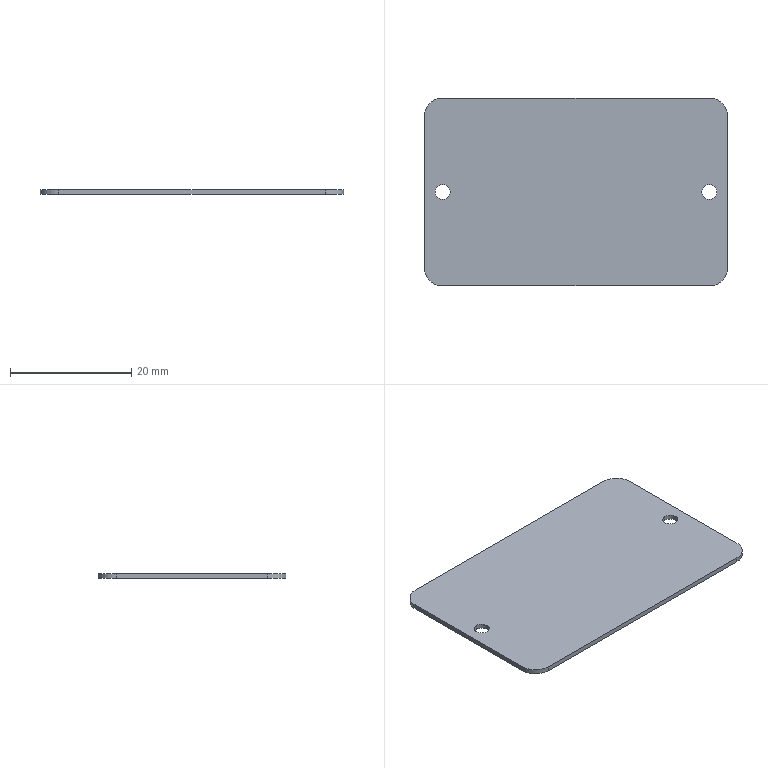Part | STEP file | Grease nameplate-Part-2 | 1 solid | 14 faces | box 50 x 31 x 0.8 mm | volume 1226 mm3 | cylinder 8 | plane 6 | commonest cylinder face diameters 2.5 x4 6 x4
STEP:
#1=CARTESIAN_POINT('',(0.,0.,0.));
#2=DIRECTION('',(0.,0.,1.));
#3=DIRECTION('',(1.,0.,0.));
#4=AXIS2_PLACEMENT_3D('',#1,#2,#3);
#5=CARTESIAN_POINT('',(47.,-16.75,0.8));
#6=VERTEX_POINT('',#5);
#7=CARTESIAN_POINT('',(47.,-16.75,0.));
#8=VERTEX_POINT('',#7);
#9=CARTESIAN_POINT('',(47.,-16.75,0.8));
#10=DIRECTION('',(0.,0.,-1.));
#11=VECTOR('',#10,1.);
#12=LINE('',#9,#11);
#13=CARTESIAN_POINT('',(47.,-15.5,0.8));
#14=DIRECTION('',(0.,0.,-1.));
#15=DIRECTION('',(0.,-1.,0.));
#16=AXIS2_PLACEMENT_3D('',#13,#14,#15);
#17=CYLINDRICAL_SURFACE('',#16,1.25);
#18=CARTESIAN_POINT('',(6.283,0.));
#19=DIRECTION('',(0.,1.));
#20=VECTOR('',#19,1.);
#21=LINE('',#18,#20);
#22=(GEOMETRIC_REPRESENTATION_CONTEXT(2)PARAMETRIC_REPRESENTATION_CONTEXT()REPRESENTATION_CONTEXT('',''));
#23=DEFINITIONAL_REPRESENTATION('',(#21),#22);
#24=PCURVE('',#17,#23);
#25=CARTESIAN_POINT('',(47.,-15.5,0.8));
#26=DIRECTION('',(0.,0.,-1.));
#27=DIRECTION('',(0.,-1.,0.));
#28=AXIS2_PLACEMENT_3D('',#25,#26,#27);
#29=CYLINDRICAL_SURFACE('',#28,1.25);
#30=CARTESIAN_POINT('',(0.,0.));
#31=DIRECTION('',(0.,1.));
#32=VECTOR('',#31,1.);
#33=LINE('',#30,#32);
#34=(GEOMETRIC_REPRESENTATION_CONTEXT(2)PARAMETRIC_REPRESENTATION_CONTEXT()REPRESENTATION_CONTEXT('',''));
#35=DEFINITIONAL_REPRESENTATION('',(#33),#34);
#36=PCURVE('',#29,#35);
#37=SURFACE_CURVE('',#12,(#24,#36),.PCURVE_S1.);
#38=EDGE_CURVE('',#6,#8,#37,.T.);
#39=ORIENTED_EDGE('',*,*,#38,.T.);
#40=CARTESIAN_POINT('',(47.,-14.25,0.));
#41=VERTEX_POINT('',#40);
#42=CARTESIAN_POINT('',(47.,-15.5,0.));
#43=DIRECTION('',(0.,0.,-1.));
#44=DIRECTION('',(0.,1.,0.));
#45=AXIS2_PLACEMENT_3D('',#42,#43,#44);
#46=CIRCLE('',#45,1.25);
#47=CARTESIAN_POINT('',(3.142,0.8));
#48=DIRECTION('',(1.,0.));
#49=VECTOR('',#48,1.);
#50=LINE('',#47,#49);
#51=(GEOMETRIC_REPRESENTATION_CONTEXT(2)PARAMETRIC_REPRESENTATION_CONTEXT()REPRESENTATION_CONTEXT('',''));
#52=DEFINITIONAL_REPRESENTATION('',(#50),#51);
#53=PCURVE('',#17,#52);
#54=CARTESIAN_POINT('',(25.,0.,0.));
#55=DIRECTION('',(0.,0.,-1.));
#56=DIRECTION('',(0.,-1.,0.));
#57=AXIS2_PLACEMENT_3D('',#54,#55,#56);
#58=PLANE('',#57);
#59=CARTESIAN_POINT('',(15.5,-22.));
#60=DIRECTION('',(-1.,0.));
#61=AXIS2_PLACEMENT_2D('',#59,#60);
#62=CIRCLE('',#61,1.25);
#63=(GEOMETRIC_REPRESENTATION_CONTEXT(2)PARAMETRIC_REPRESENTATION_CONTEXT()REPRESENTATION_CONTEXT('',''));
#64=DEFINITIONAL_REPRESENTATION('',(#62),#63);
#65=PCURVE('',#58,#64);
#66=SURFACE_CURVE('',#46,(#53,#65),.PCURVE_S1.);
#67=EDGE_CURVE('',#41,#8,#66,.T.);
#68=ORIENTED_EDGE('',*,*,#67,.F.);
#69=CARTESIAN_POINT('',(47.,-14.25,0.8));
#70=VERTEX_POINT('',#69);
#71=CARTESIAN_POINT('',(47.,-14.25,0.8));
#72=DIRECTION('',(0.,0.,-1.));
#73=VECTOR('',#72,1.);
#74=LINE('',#71,#73);
#75=CARTESIAN_POINT('',(3.142,0.));
#76=DIRECTION('',(0.,1.));
#77=VECTOR('',#76,1.);
#78=LINE('',#75,#77);
#79=(GEOMETRIC_REPRESENTATION_CONTEXT(2)PARAMETRIC_REPRESENTATION_CONTEXT()REPRESENTATION_CONTEXT('',''));
#80=DEFINITIONAL_REPRESENTATION('',(#78),#79);
#81=PCURVE('',#17,#80);
#82=CARTESIAN_POINT('',(3.142,0.));
#83=DIRECTION('',(0.,1.));
#84=VECTOR('',#83,1.);
#85=LINE('',#82,#84);
#86=(GEOMETRIC_REPRESENTATION_CONTEXT(2)PARAMETRIC_REPRESENTATION_CONTEXT()REPRESENTATION_CONTEXT('',''));
#87=DEFINITIONAL_REPRESENTATION('',(#85),#86);
#88=PCURVE('',#29,#87);
#89=SURFACE_CURVE('',#74,(#81,#88),.PCURVE_S1.);
#90=EDGE_CURVE('',#70,#41,#89,.T.);
#91=ORIENTED_EDGE('',*,*,#90,.F.);
#92=CARTESIAN_POINT('',(47.,-15.5,0.8));
#93=DIRECTION('',(0.,0.,1.));
#94=DIRECTION('',(0.,-1.,0.));
#95=AXIS2_PLACEMENT_3D('',#92,#93,#94);
#96=CIRCLE('',#95,1.25);
#97=CARTESIAN_POINT('',(6.283,0.));
#98=DIRECTION('',(-1.,0.));
#99=VECTOR('',#98,1.);
#100=LINE('',#97,#99);
#101=(GEOMETRIC_REPRESENTATION_CONTEXT(2)PARAMETRIC_REPRESENTATION_CONTEXT()REPRESENTATION_CONTEXT('',''));
#102=DEFINITIONAL_REPRESENTATION('',(#100),#101);
#103=PCURVE('',#17,#102);
#104=CARTESIAN_POINT('',(25.,0.,0.8));
#105=DIRECTION('',(0.,0.,1.));
#106=DIRECTION('',(0.,1.,0.));
#107=AXIS2_PLACEMENT_3D('',#104,#105,#106);
#108=PLANE('',#107);
#109=CARTESIAN_POINT('',(-15.5,-22.));
#110=DIRECTION('',(-1.,0.));
#111=AXIS2_PLACEMENT_2D('',#109,#110);
#112=CIRCLE('',#111,1.25);
#113=(GEOMETRIC_REPRESENTATION_CONTEXT(2)PARAMETRIC_REPRESENTATION_CONTEXT()REPRESENTATION_CONTEXT('',''));
#114=DEFINITIONAL_REPRESENTATION('',(#112),#113);
#115=PCURVE('',#108,#114);
#116=SURFACE_CURVE('',#96,(#103,#115),.PCURVE_S1.);
#117=EDGE_CURVE('',#6,#70,#116,.T.);
#118=ORIENTED_EDGE('',*,*,#117,.F.);
#119=EDGE_LOOP('',(#39,#68,#91,#118));
#120=FACE_BOUND('',#119,.F.);
#121=ADVANCED_FACE('',(#120),#17,.F.);
#122=CARTESIAN_POINT('',(3.,-16.75,0.8));
#123=VERTEX_POINT('',#122);
#124=CARTESIAN_POINT('',(3.,-16.75,0.));
#125=VERTEX_POINT('',#124);
#126=CARTESIAN_POINT('',(3.,-16.75,0.8));
#127=DIRECTION('',(0.,0.,-1.));
#128=VECTOR('',#127,1.);
#129=LINE('',#126,#128);
#130=CARTESIAN_POINT('',(3.,-15.5,0.8));
#131=DIRECTION('',(0.,0.,-1.));
#132=DIRECTION('',(0.,-1.,0.));
#133=AXIS2_PLACEMENT_3D('',#130,#131,#132);
#134=CYLINDRICAL_SURFACE('',#133,1.25);
#135=CARTESIAN_POINT('',(6.283,0.));
#136=DIRECTION('',(0.,1.));
#137=VECTOR('',#136,1.);
#138=LINE('',#135,#137);
#139=(GEOMETRIC_REPRESENTATION_CONTEXT(2)PARAMETRIC_REPRESENTATION_CONTEXT()REPRESENTATION_CONTEXT('',''));
#140=DEFINITIONAL_REPRESENTATION('',(#138),#139);
#141=PCURVE('',#134,#140);
#142=CARTESIAN_POINT('',(3.,-15.5,0.8));
#143=DIRECTION('',(0.,0.,-1.));
#144=DIRECTION('',(0.,-1.,0.));
#145=AXIS2_PLACEMENT_3D('',#142,#143,#144);
#146=CYLINDRICAL_SURFACE('',#145,1.25);
#147=CARTESIAN_POINT('',(0.,0.));
#148=DIRECTION('',(0.,1.));
#149=VECTOR('',#148,1.);
#150=LINE('',#147,#149);
#151=(GEOMETRIC_REPRESENTATION_CONTEXT(2)PARAMETRIC_REPRESENTATION_CONTEXT()REPRESENTATION_CONTEXT('',''));
#152=DEFINITIONAL_REPRESENTATION('',(#150),#151);
#153=PCURVE('',#146,#152);
#154=SURFACE_CURVE('',#129,(#141,#153),.PCURVE_S1.);
#155=EDGE_CURVE('',#123,#125,#154,.T.);
#156=ORIENTED_EDGE('',*,*,#155,.T.);
#157=CARTESIAN_POINT('',(3.,-14.25,0.));
#158=VERTEX_POINT('',#157);
#159=CARTESIAN_POINT('',(3.,-15.5,0.));
#160=DIRECTION('',(0.,0.,-1.));
#161=DIRECTION('',(0.,1.,0.));
#162=AXIS2_PLACEMENT_3D('',#159,#160,#161);
#163=CIRCLE('',#162,1.25);
#164=CARTESIAN_POINT('',(3.142,0.8));
#165=DIRECTION('',(1.,0.));
#166=VECTOR('',#165,1.);
#167=LINE('',#164,#166);
#168=(GEOMETRIC_REPRESENTATION_CONTEXT(2)PARAMETRIC_REPRESENTATION_CONTEXT()REPRESENTATION_CONTEXT('',''));
#169=DEFINITIONAL_REPRESENTATION('',(#167),#168);
#170=PCURVE('',#134,#169);
#171=CARTESIAN_POINT('',(15.5,22.));
#172=DIRECTION('',(-1.,0.));
#173=AXIS2_PLACEMENT_2D('',#171,#172);
#174=CIRCLE('',#173,1.25);
#175=(GEOMETRIC_REPRESENTATION_CONTEXT(2)PARAMETRIC_REPRESENTATION_CONTEXT()REPRESENTATION_CONTEXT('',''));
#176=DEFINITIONAL_REPRESENTATION('',(#174),#175);
#177=PCURVE('',#58,#176);
#178=SURFACE_CURVE('',#163,(#170,#177),.PCURVE_S1.);
#179=EDGE_CURVE('',#158,#125,#178,.T.);
#180=ORIENTED_EDGE('',*,*,#179,.F.);
#181=CARTESIAN_POINT('',(3.,-14.25,0.8));
#182=VERTEX_POINT('',#181);
#183=CARTESIAN_POINT('',(3.,-14.25,0.8));
#184=DIRECTION('',(0.,0.,-1.));
#185=VECTOR('',#184,1.);
#186=LINE('',#183,#185);
#187=CARTESIAN_POINT('',(3.142,0.));
#188=DIRECTION('',(0.,1.));
#189=VECTOR('',#188,1.);
#190=LINE('',#187,#189);
#191=(GEOMETRIC_REPRESENTATION_CONTEXT(2)PARAMETRIC_REPRESENTATION_CONTEXT()REPRESENTATION_CONTEXT('',''));
#192=DEFINITIONAL_REPRESENTATION('',(#190),#191);
#193=PCURVE('',#134,#192);
#194=CARTESIAN_POINT('',(3.142,0.));
#195=DIRECTION('',(0.,1.));
#196=VECTOR('',#195,1.);
#197=LINE('',#194,#196);
#198=(GEOMETRIC_REPRESENTATION_CONTEXT(2)PARAMETRIC_REPRESENTATION_CONTEXT()REPRESENTATION_CONTEXT('',''));
#199=DEFINITIONAL_REPRESENTATION('',(#197),#198);
#200=PCURVE('',#146,#199);
#201=SURFACE_CURVE('',#186,(#193,#200),.PCURVE_S1.);
#202=EDGE_CURVE('',#182,#158,#201,.T.);
#203=ORIENTED_EDGE('',*,*,#202,.F.);
#204=CARTESIAN_POINT('',(3.,-15.5,0.8));
#205=DIRECTION('',(0.,0.,1.));
#206=DIRECTION('',(0.,-1.,0.));
#207=AXIS2_PLACEMENT_3D('',#204,#205,#206);
#208=CIRCLE('',#207,1.25);
#209=CARTESIAN_POINT('',(6.283,0.));
#210=DIRECTION('',(-1.,0.));
#211=VECTOR('',#210,1.);
#212=LINE('',#209,#211);
#213=(GEOMETRIC_REPRESENTATION_CONTEXT(2)PARAMETRIC_REPRESENTATION_CONTEXT()REPRESENTATION_CONTEXT('',''));
#214=DEFINITIONAL_REPRESENTATION('',(#212),#213);
#215=PCURVE('',#134,#214);
#216=CARTESIAN_POINT('',(-15.5,22.));
#217=DIRECTION('',(-1.,0.));
#218=AXIS2_PLACEMENT_2D('',#216,#217);
#219=CIRCLE('',#218,1.25);
#220=(GEOMETRIC_REPRESENTATION_CONTEXT(2)PARAMETRIC_REPRESENTATION_CONTEXT()REPRESENTATION_CONTEXT('',''));
#221=DEFINITIONAL_REPRESENTATION('',(#219),#220);
#222=PCURVE('',#108,#221);
#223=SURFACE_CURVE('',#208,(#215,#222),.PCURVE_S1.);
#224=EDGE_CURVE('',#123,#182,#223,.T.);
#225=ORIENTED_EDGE('',*,*,#224,.F.);
#226=EDGE_LOOP('',(#156,#180,#203,#225));
#227=FACE_BOUND('',#226,.F.);
#228=ADVANCED_FACE('',(#227),#134,.F.);
#229=CARTESIAN_POINT('',(3.,-31.,0.));
#230=VERTEX_POINT('',#229);
#231=CARTESIAN_POINT('',(47.,-31.,0.));
#232=VERTEX_POINT('',#231);
#233=CARTESIAN_POINT('',(25.,-31.,0.));
#234=DIRECTION('',(1.,0.,0.));
#235=VECTOR('',#234,1.);
#236=LINE('',#233,#235);
#237=CARTESIAN_POINT('',(25.,-31.,0.4));
#238=DIRECTION('',(0.,-1.,0.));
#239=DIRECTION('',(1.,0.,0.));
#240=AXIS2_PLACEMENT_3D('',#237,#238,#239);
#241=PLANE('',#240);
#242=CARTESIAN_POINT('',(0.,-0.4));
#243=DIRECTION('',(1.,0.));
#244=VECTOR('',#243,1.);
#245=LINE('',#242,#244);
#246=(GEOMETRIC_REPRESENTATION_CONTEXT(2)PARAMETRIC_REPRESENTATION_CONTEXT()REPRESENTATION_CONTEXT('',''));
#247=DEFINITIONAL_REPRESENTATION('',(#245),#246);
#248=PCURVE('',#241,#247);
#249=CARTESIAN_POINT('',(31.,0.));
#250=DIRECTION('',(0.,-1.));
#251=VECTOR('',#250,1.);
#252=LINE('',#249,#251);
#253=(GEOMETRIC_REPRESENTATION_CONTEXT(2)PARAMETRIC_REPRESENTATION_CONTEXT()REPRESENTATION_CONTEXT('',''));
#254=DEFINITIONAL_REPRESENTATION('',(#252),#253);
#255=PCURVE('',#58,#254);
#256=SURFACE_CURVE('',#236,(#248,#255),.PCURVE_S1.);
#257=EDGE_CURVE('',#230,#232,#256,.T.);
#258=ORIENTED_EDGE('',*,*,#257,.T.);
#259=CARTESIAN_POINT('',(47.,-31.,0.8));
#260=VERTEX_POINT('',#259);
#261=CARTESIAN_POINT('',(47.,-31.,0.4));
#262=DIRECTION('',(0.,0.,-1.));
#263=VECTOR('',#262,1.);
#264=LINE('',#261,#263);
#265=CARTESIAN_POINT('',(22.,0.));
#266=DIRECTION('',(0.,-1.));
#267=VECTOR('',#266,1.);
#268=LINE('',#265,#267);
#269=(GEOMETRIC_REPRESENTATION_CONTEXT(2)PARAMETRIC_REPRESENTATION_CONTEXT()REPRESENTATION_CONTEXT('',''));
#270=DEFINITIONAL_REPRESENTATION('',(#268),#269);
#271=PCURVE('',#241,#270);
#272=CARTESIAN_POINT('',(47.,-28.,0.4));
#273=DIRECTION('',(0.,0.,1.));
#274=DIRECTION('',(0.,1.,0.));
#275=AXIS2_PLACEMENT_3D('',#272,#273,#274);
#276=CYLINDRICAL_SURFACE('',#275,3.);
#277=CARTESIAN_POINT('',(3.142,0.));
#278=DIRECTION('',(0.,-1.));
#279=VECTOR('',#278,1.);
#280=LINE('',#277,#279);
#281=(GEOMETRIC_REPRESENTATION_CONTEXT(2)PARAMETRIC_REPRESENTATION_CONTEXT()REPRESENTATION_CONTEXT('',''));
#282=DEFINITIONAL_REPRESENTATION('',(#280),#281);
#283=PCURVE('',#276,#282);
#284=SURFACE_CURVE('',#264,(#271,#283),.PCURVE_S1.);
#285=EDGE_CURVE('',#260,#232,#284,.T.);
#286=ORIENTED_EDGE('',*,*,#285,.F.);
#287=CARTESIAN_POINT('',(3.,-31.,0.8));
#288=VERTEX_POINT('',#287);
#289=CARTESIAN_POINT('',(25.,-31.,0.8));
#290=DIRECTION('',(-1.,0.,0.));
#291=VECTOR('',#290,1.);
#292=LINE('',#289,#291);
#293=CARTESIAN_POINT('',(0.,0.4));
#294=DIRECTION('',(-1.,0.));
#295=VECTOR('',#294,1.);
#296=LINE('',#293,#295);
#297=(GEOMETRIC_REPRESENTATION_CONTEXT(2)PARAMETRIC_REPRESENTATION_CONTEXT()REPRESENTATION_CONTEXT('',''));
#298=DEFINITIONAL_REPRESENTATION('',(#296),#297);
#299=PCURVE('',#241,#298);
#300=CARTESIAN_POINT('',(-31.,0.));
#301=DIRECTION('',(0.,1.));
#302=VECTOR('',#301,1.);
#303=LINE('',#300,#302);
#304=(GEOMETRIC_REPRESENTATION_CONTEXT(2)PARAMETRIC_REPRESENTATION_CONTEXT()REPRESENTATION_CONTEXT('',''));
#305=DEFINITIONAL_REPRESENTATION('',(#303),#304);
#306=PCURVE('',#108,#305);
#307=SURFACE_CURVE('',#292,(#299,#306),.PCURVE_S1.);
#308=EDGE_CURVE('',#260,#288,#307,.T.);
#309=ORIENTED_EDGE('',*,*,#308,.T.);
#310=CARTESIAN_POINT('',(3.,-31.,0.4));
#311=DIRECTION('',(0.,0.,1.));
#312=VECTOR('',#311,1.);
#313=LINE('',#310,#312);
#314=CARTESIAN_POINT('',(-22.,0.));
#315=DIRECTION('',(0.,1.));
#316=VECTOR('',#315,1.);
#317=LINE('',#314,#316);
#318=(GEOMETRIC_REPRESENTATION_CONTEXT(2)PARAMETRIC_REPRESENTATION_CONTEXT()REPRESENTATION_CONTEXT('',''));
#319=DEFINITIONAL_REPRESENTATION('',(#317),#318);
#320=PCURVE('',#241,#319);
#321=CARTESIAN_POINT('',(3.,-28.,0.4));
#322=DIRECTION('',(0.,0.,-1.));
#323=DIRECTION('',(0.,-1.,0.));
#324=AXIS2_PLACEMENT_3D('',#321,#322,#323);
#325=CYLINDRICAL_SURFACE('',#324,3.);
#326=CARTESIAN_POINT('',(0.,0.));
#327=DIRECTION('',(0.,-1.));
#328=VECTOR('',#327,1.);
#329=LINE('',#326,#328);
#330=(GEOMETRIC_REPRESENTATION_CONTEXT(2)PARAMETRIC_REPRESENTATION_CONTEXT()REPRESENTATION_CONTEXT('',''));
#331=DEFINITIONAL_REPRESENTATION('',(#329),#330);
#332=PCURVE('',#325,#331);
#333=SURFACE_CURVE('',#313,(#320,#332),.PCURVE_S1.);
#334=EDGE_CURVE('',#230,#288,#333,.T.);
#335=ORIENTED_EDGE('',*,*,#334,.F.);
#336=EDGE_LOOP('',(#258,#286,#309,#335));
#337=FACE_BOUND('',#336,.T.);
#338=ADVANCED_FACE('',(#337),#241,.T.);
#339=ORIENTED_EDGE('',*,*,#117,.F.);
#340=CARTESIAN_POINT('',(47.,-15.5,0.8));
#341=DIRECTION('',(0.,0.,1.));
#342=DIRECTION('',(0.,-1.,0.));
#343=AXIS2_PLACEMENT_3D('',#340,#341,#342);
#344=CIRCLE('',#343,1.25);
#345=CARTESIAN_POINT('',(-15.5,-22.));
#346=DIRECTION('',(-1.,0.));
#347=AXIS2_PLACEMENT_2D('',#345,#346);
#348=CIRCLE('',#347,1.25);
#349=(GEOMETRIC_REPRESENTATION_CONTEXT(2)PARAMETRIC_REPRESENTATION_CONTEXT()REPRESENTATION_CONTEXT('',''));
#350=DEFINITIONAL_REPRESENTATION('',(#348),#349);
#351=PCURVE('',#108,#350);
#352=CARTESIAN_POINT('',(6.283,0.));
#353=DIRECTION('',(-1.,0.));
#354=VECTOR('',#353,1.);
#355=LINE('',#352,#354);
#356=(GEOMETRIC_REPRESENTATION_CONTEXT(2)PARAMETRIC_REPRESENTATION_CONTEXT()REPRESENTATION_CONTEXT('',''));
#357=DEFINITIONAL_REPRESENTATION('',(#355),#356);
#358=PCURVE('',#29,#357);
#359=SURFACE_CURVE('',#344,(#351,#358),.PCURVE_S1.);
#360=EDGE_CURVE('',#70,#6,#359,.T.);
#361=ORIENTED_EDGE('',*,*,#360,.F.);
#362=EDGE_LOOP('',(#339,#361));
#363=FACE_BOUND('',#362,.T.);
#364=ORIENTED_EDGE('',*,*,#224,.F.);
#365=CARTESIAN_POINT('',(3.,-15.5,0.8));
#366=DIRECTION('',(0.,0.,1.));
#367=DIRECTION('',(0.,-1.,0.));
#368=AXIS2_PLACEMENT_3D('',#365,#366,#367);
#369=CIRCLE('',#368,1.25);
#370=CARTESIAN_POINT('',(-15.5,22.));
#371=DIRECTION('',(-1.,0.));
#372=AXIS2_PLACEMENT_2D('',#370,#371);
#373=CIRCLE('',#372,1.25);
#374=(GEOMETRIC_REPRESENTATION_CONTEXT(2)PARAMETRIC_REPRESENTATION_CONTEXT()REPRESENTATION_CONTEXT('',''));
#375=DEFINITIONAL_REPRESENTATION('',(#373),#374);
#376=PCURVE('',#108,#375);
#377=CARTESIAN_POINT('',(6.283,0.));
#378=DIRECTION('',(-1.,0.));
#379=VECTOR('',#378,1.);
#380=LINE('',#377,#379);
#381=(GEOMETRIC_REPRESENTATION_CONTEXT(2)PARAMETRIC_REPRESENTATION_CONTEXT()REPRESENTATION_CONTEXT('',''));
#382=DEFINITIONAL_REPRESENTATION('',(#380),#381);
#383=PCURVE('',#146,#382);
#384=SURFACE_CURVE('',#369,(#376,#383),.PCURVE_S1.);
#385=EDGE_CURVE('',#182,#123,#384,.T.);
#386=ORIENTED_EDGE('',*,*,#385,.F.);
#387=EDGE_LOOP('',(#364,#386));
#388=FACE_BOUND('',#387,.T.);
#389=CARTESIAN_POINT('',(0.,-3.,0.8));
#390=VERTEX_POINT('',#389);
#391=CARTESIAN_POINT('',(0.,-28.,0.8));
#392=VERTEX_POINT('',#391);
#393=CARTESIAN_POINT('',(0.,0.,0.8));
#394=DIRECTION('',(0.,-1.,0.));
#395=VECTOR('',#394,1.);
#396=LINE('',#393,#395);
#397=CARTESIAN_POINT('',(0.,25.));
#398=DIRECTION('',(-1.,0.));
#399=VECTOR('',#398,1.);
#400=LINE('',#397,#399);
#401=(GEOMETRIC_REPRESENTATION_CONTEXT(2)PARAMETRIC_REPRESENTATION_CONTEXT()REPRESENTATION_CONTEXT('',''));
#402=DEFINITIONAL_REPRESENTATION('',(#400),#401);
#403=PCURVE('',#108,#402);
#404=CARTESIAN_POINT('',(0.,0.,0.4));
#405=DIRECTION('',(-1.,0.,0.));
#406=DIRECTION('',(0.,-1.,0.));
#407=AXIS2_PLACEMENT_3D('',#404,#405,#406);
#408=PLANE('',#407);
#409=CARTESIAN_POINT('',(0.,0.4));
#410=DIRECTION('',(1.,0.));
#411=VECTOR('',#410,1.);
#412=LINE('',#409,#411);
#413=(GEOMETRIC_REPRESENTATION_CONTEXT(2)PARAMETRIC_REPRESENTATION_CONTEXT()REPRESENTATION_CONTEXT('',''));
#414=DEFINITIONAL_REPRESENTATION('',(#412),#413);
#415=PCURVE('',#408,#414);
#416=SURFACE_CURVE('',#396,(#403,#415),.PCURVE_S1.);
#417=EDGE_CURVE('',#390,#392,#416,.T.);
#418=ORIENTED_EDGE('',*,*,#417,.T.);
#419=CARTESIAN_POINT('',(3.,-28.,0.8));
#420=DIRECTION('',(0.,0.,-1.));
#421=DIRECTION('',(0.,1.,0.));
#422=AXIS2_PLACEMENT_3D('',#419,#420,#421);
#423=CIRCLE('',#422,3.);
#424=CARTESIAN_POINT('',(-25.,22.));
#425=CARTESIAN_POINT('',(-25.,16.804));
#426=CARTESIAN_POINT('',(-29.5,19.402));
#427=CARTESIAN_POINT('',(-34.,22.));
#428=CARTESIAN_POINT('',(-29.5,24.598));
#429=CARTESIAN_POINT('',(-25.,27.196));
#430=CARTESIAN_POINT('',(-25.,22.));
#431=(BOUNDED_CURVE()B_SPLINE_CURVE(2,(#424,#425,#426,#427,#428,#429,#430),.UNSPECIFIED.,.T.,.F.)B_SPLINE_CURVE_WITH_KNOTS((1,2,2,2,2,1),(-2.094,0.,2.094,4.189,6.283,8.378),.UNSPECIFIED.)CURVE()GEOMETRIC_REPRESENTATION_ITEM()RATIONAL_B_SPLINE_CURVE((1.,0.5,1.,0.5,1.,0.5,1.))REPRESENTATION_ITEM(''));
#432=(GEOMETRIC_REPRESENTATION_CONTEXT(2)PARAMETRIC_REPRESENTATION_CONTEXT()REPRESENTATION_CONTEXT('',''));
#433=DEFINITIONAL_REPRESENTATION('',(#431),#432);
#434=PCURVE('',#108,#433);
#435=CARTESIAN_POINT('',(-3.142,-0.4));
#436=DIRECTION('',(1.,0.));
#437=VECTOR('',#436,1.);
#438=LINE('',#435,#437);
#439=(GEOMETRIC_REPRESENTATION_CONTEXT(2)PARAMETRIC_REPRESENTATION_CONTEXT()REPRESENTATION_CONTEXT('',''));
#440=DEFINITIONAL_REPRESENTATION('',(#438),#439);
#441=PCURVE('',#325,#440);
#442=SURFACE_CURVE('',#423,(#434,#441),.PCURVE_S1.);
#443=EDGE_CURVE('',#288,#392,#442,.T.);
#444=ORIENTED_EDGE('',*,*,#443,.F.);
#445=ORIENTED_EDGE('',*,*,#308,.F.);
#446=CARTESIAN_POINT('',(50.,-28.,0.8));
#447=VERTEX_POINT('',#446);
#448=CARTESIAN_POINT('',(47.,-28.,0.8));
#449=DIRECTION('',(0.,0.,-1.));
#450=DIRECTION('',(0.,1.,0.));
#451=AXIS2_PLACEMENT_3D('',#448,#449,#450);
#452=CIRCLE('',#451,3.);
#453=CARTESIAN_POINT('',(-25.,-22.));
#454=CARTESIAN_POINT('',(-25.,-27.196));
#455=CARTESIAN_POINT('',(-29.5,-24.598));
#456=CARTESIAN_POINT('',(-34.,-22.));
#457=CARTESIAN_POINT('',(-29.5,-19.402));
#458=CARTESIAN_POINT('',(-25.,-16.804));
#459=CARTESIAN_POINT('',(-25.,-22.));
#460=(BOUNDED_CURVE()B_SPLINE_CURVE(2,(#453,#454,#455,#456,#457,#458,#459),.UNSPECIFIED.,.T.,.F.)B_SPLINE_CURVE_WITH_KNOTS((1,2,2,2,2,1),(-2.094,0.,2.094,4.189,6.283,8.378),.UNSPECIFIED.)CURVE()GEOMETRIC_REPRESENTATION_ITEM()RATIONAL_B_SPLINE_CURVE((1.,0.5,1.,0.5,1.,0.5,1.))REPRESENTATION_ITEM(''));
#461=(GEOMETRIC_REPRESENTATION_CONTEXT(2)PARAMETRIC_REPRESENTATION_CONTEXT()REPRESENTATION_CONTEXT('',''));
#462=DEFINITIONAL_REPRESENTATION('',(#460),#461);
#463=PCURVE('',#108,#462);
#464=CARTESIAN_POINT('',(6.283,0.4));
#465=DIRECTION('',(-1.,0.));
#466=VECTOR('',#465,1.);
#467=LINE('',#464,#466);
#468=(GEOMETRIC_REPRESENTATION_CONTEXT(2)PARAMETRIC_REPRESENTATION_CONTEXT()REPRESENTATION_CONTEXT('',''));
#469=DEFINITIONAL_REPRESENTATION('',(#467),#468);
#470=PCURVE('',#276,#469);
#471=SURFACE_CURVE('',#452,(#463,#470),.PCURVE_S1.);
#472=EDGE_CURVE('',#447,#260,#471,.T.);
#473=ORIENTED_EDGE('',*,*,#472,.F.);
#474=CARTESIAN_POINT('',(50.,-3.,0.8));
#475=VERTEX_POINT('',#474);
#476=CARTESIAN_POINT('',(50.,0.,0.8));
#477=DIRECTION('',(0.,-1.,0.));
#478=VECTOR('',#477,1.);
#479=LINE('',#476,#478);
#480=CARTESIAN_POINT('',(0.,-25.));
#481=DIRECTION('',(-1.,0.));
#482=VECTOR('',#481,1.);
#483=LINE('',#480,#482);
#484=(GEOMETRIC_REPRESENTATION_CONTEXT(2)PARAMETRIC_REPRESENTATION_CONTEXT()REPRESENTATION_CONTEXT('',''));
#485=DEFINITIONAL_REPRESENTATION('',(#483),#484);
#486=PCURVE('',#108,#485);
#487=CARTESIAN_POINT('',(50.,0.,0.4));
#488=DIRECTION('',(1.,0.,0.));
#489=DIRECTION('',(0.,1.,0.));
#490=AXIS2_PLACEMENT_3D('',#487,#488,#489);
#491=PLANE('',#490);
#492=CARTESIAN_POINT('',(0.,0.4));
#493=DIRECTION('',(-1.,0.));
#494=VECTOR('',#493,1.);
#495=LINE('',#492,#494);
#496=(GEOMETRIC_REPRESENTATION_CONTEXT(2)PARAMETRIC_REPRESENTATION_CONTEXT()REPRESENTATION_CONTEXT('',''));
#497=DEFINITIONAL_REPRESENTATION('',(#495),#496);
#498=PCURVE('',#491,#497);
#499=SURFACE_CURVE('',#479,(#486,#498),.PCURVE_S1.);
#500=EDGE_CURVE('',#475,#447,#499,.T.);
#501=ORIENTED_EDGE('',*,*,#500,.F.);
#502=CARTESIAN_POINT('',(47.,0.,0.8));
#503=VERTEX_POINT('',#502);
#504=CARTESIAN_POINT('',(47.,-3.,0.8));
#505=DIRECTION('',(0.,0.,-1.));
#506=DIRECTION('',(0.,1.,0.));
#507=AXIS2_PLACEMENT_3D('',#504,#505,#506);
#508=CIRCLE('',#507,3.);
#509=CARTESIAN_POINT('',(0.,-22.));
#510=CARTESIAN_POINT('',(0.,-27.196));
#511=CARTESIAN_POINT('',(-4.5,-24.598));
#512=CARTESIAN_POINT('',(-9.,-22.));
#513=CARTESIAN_POINT('',(-4.5,-19.402));
#514=CARTESIAN_POINT('',(0.,-16.804));
#515=CARTESIAN_POINT('',(0.,-22.));
#516=(BOUNDED_CURVE()B_SPLINE_CURVE(2,(#509,#510,#511,#512,#513,#514,#515),.UNSPECIFIED.,.T.,.F.)B_SPLINE_CURVE_WITH_KNOTS((1,2,2,2,2,1),(-2.094,0.,2.094,4.189,6.283,8.378),.UNSPECIFIED.)CURVE()GEOMETRIC_REPRESENTATION_ITEM()RATIONAL_B_SPLINE_CURVE((1.,0.5,1.,0.5,1.,0.5,1.))REPRESENTATION_ITEM(''));
#517=(GEOMETRIC_REPRESENTATION_CONTEXT(2)PARAMETRIC_REPRESENTATION_CONTEXT()REPRESENTATION_CONTEXT('',''));
#518=DEFINITIONAL_REPRESENTATION('',(#516),#517);
#519=PCURVE('',#108,#518);
#520=CARTESIAN_POINT('',(47.,-3.,0.4));
#521=DIRECTION('',(0.,0.,-1.));
#522=DIRECTION('',(0.,-1.,0.));
#523=AXIS2_PLACEMENT_3D('',#520,#521,#522);
#524=CYLINDRICAL_SURFACE('',#523,3.);
#525=CARTESIAN_POINT('',(3.142,-0.4));
#526=DIRECTION('',(1.,0.));
#527=VECTOR('',#526,1.);
#528=LINE('',#525,#527);
#529=(GEOMETRIC_REPRESENTATION_CONTEXT(2)PARAMETRIC_REPRESENTATION_CONTEXT()REPRESENTATION_CONTEXT('',''));
#530=DEFINITIONAL_REPRESENTATION('',(#528),#529);
#531=PCURVE('',#524,#530);
#532=SURFACE_CURVE('',#508,(#519,#531),.PCURVE_S1.);
#533=EDGE_CURVE('',#503,#475,#532,.T.);
#534=ORIENTED_EDGE('',*,*,#533,.F.);
#535=CARTESIAN_POINT('',(3.,0.,0.8));
#536=VERTEX_POINT('',#535);
#537=CARTESIAN_POINT('',(25.,0.,0.8));
#538=DIRECTION('',(1.,0.,0.));
#539=VECTOR('',#538,1.);
#540=LINE('',#537,#539);
#541=CARTESIAN_POINT('',(0.,0.));
#542=DIRECTION('',(0.,-1.));
#543=VECTOR('',#542,1.);
#544=LINE('',#541,#543);
#545=(GEOMETRIC_REPRESENTATION_CONTEXT(2)PARAMETRIC_REPRESENTATION_CONTEXT()REPRESENTATION_CONTEXT('',''));
#546=DEFINITIONAL_REPRESENTATION('',(#544),#545);
#547=PCURVE('',#108,#546);
#548=CARTESIAN_POINT('',(25.,0.,0.4));
#549=DIRECTION('',(0.,1.,0.));
#550=DIRECTION('',(-1.,0.,0.));
#551=AXIS2_PLACEMENT_3D('',#548,#549,#550);
#552=PLANE('',#551);
#553=CARTESIAN_POINT('',(0.,0.4));
#554=DIRECTION('',(-1.,0.));
#555=VECTOR('',#554,1.);
#556=LINE('',#553,#555);
#557=(GEOMETRIC_REPRESENTATION_CONTEXT(2)PARAMETRIC_REPRESENTATION_CONTEXT()REPRESENTATION_CONTEXT('',''));
#558=DEFINITIONAL_REPRESENTATION('',(#556),#557);
#559=PCURVE('',#552,#558);
#560=SURFACE_CURVE('',#540,(#547,#559),.PCURVE_S1.);
#561=EDGE_CURVE('',#536,#503,#560,.T.);
#562=ORIENTED_EDGE('',*,*,#561,.F.);
#563=CARTESIAN_POINT('',(3.,-3.,0.8));
#564=DIRECTION('',(0.,0.,-1.));
#565=DIRECTION('',(0.,1.,0.));
#566=AXIS2_PLACEMENT_3D('',#563,#564,#565);
#567=CIRCLE('',#566,3.);
#568=CARTESIAN_POINT('',(0.,22.));
#569=CARTESIAN_POINT('',(0.,16.804));
#570=CARTESIAN_POINT('',(-4.5,19.402));
#571=CARTESIAN_POINT('',(-9.,22.));
#572=CARTESIAN_POINT('',(-4.5,24.598));
#573=CARTESIAN_POINT('',(0.,27.196));
#574=CARTESIAN_POINT('',(0.,22.));
#575=(BOUNDED_CURVE()B_SPLINE_CURVE(2,(#568,#569,#570,#571,#572,#573,#574),.UNSPECIFIED.,.T.,.F.)B_SPLINE_CURVE_WITH_KNOTS((1,2,2,2,2,1),(-2.094,0.,2.094,4.189,6.283,8.378),.UNSPECIFIED.)CURVE()GEOMETRIC_REPRESENTATION_ITEM()RATIONAL_B_SPLINE_CURVE((1.,0.5,1.,0.5,1.,0.5,1.))REPRESENTATION_ITEM(''));
#576=(GEOMETRIC_REPRESENTATION_CONTEXT(2)PARAMETRIC_REPRESENTATION_CONTEXT()REPRESENTATION_CONTEXT('',''));
#577=DEFINITIONAL_REPRESENTATION('',(#575),#576);
#578=PCURVE('',#108,#577);
#579=CARTESIAN_POINT('',(3.,-3.,0.4));
#580=DIRECTION('',(0.,0.,1.));
#581=DIRECTION('',(0.,1.,0.));
#582=AXIS2_PLACEMENT_3D('',#579,#580,#581);
#583=CYLINDRICAL_SURFACE('',#582,3.);
#584=CARTESIAN_POINT('',(6.283,0.4));
#585=DIRECTION('',(-1.,0.));
#586=VECTOR('',#585,1.);
#587=LINE('',#584,#586);
#588=(GEOMETRIC_REPRESENTATION_CONTEXT(2)PARAMETRIC_REPRESENTATION_CONTEXT()REPRESENTATION_CONTEXT('',''));
#589=DEFINITIONAL_REPRESENTATION('',(#587),#588);
#590=PCURVE('',#583,#589);
#591=SURFACE_CURVE('',#567,(#578,#590),.PCURVE_S1.);
#592=EDGE_CURVE('',#390,#536,#591,.T.);
#593=ORIENTED_EDGE('',*,*,#592,.F.);
#594=EDGE_LOOP('',(#418,#444,#445,#473,#501,#534,#562,#593));
#595=FACE_BOUND('',#594,.T.);
#596=ADVANCED_FACE('',(#363,#388,#595),#108,.T.);
#597=CARTESIAN_POINT('',(0.,-3.,0.));
#598=VERTEX_POINT('',#597);
#599=CARTESIAN_POINT('',(0.,-28.,0.));
#600=VERTEX_POINT('',#599);
#601=CARTESIAN_POINT('',(0.,0.,0.));
#602=DIRECTION('',(0.,-1.,0.));
#603=VECTOR('',#602,1.);
#604=LINE('',#601,#603);
#605=CARTESIAN_POINT('',(0.,-0.4));
#606=DIRECTION('',(1.,0.));
#607=VECTOR('',#606,1.);
#608=LINE('',#605,#607);
#609=(GEOMETRIC_REPRESENTATION_CONTEXT(2)PARAMETRIC_REPRESENTATION_CONTEXT()REPRESENTATION_CONTEXT('',''));
#610=DEFINITIONAL_REPRESENTATION('',(#608),#609);
#611=PCURVE('',#408,#610);
#612=CARTESIAN_POINT('',(0.,25.));
#613=DIRECTION('',(1.,0.));
#614=VECTOR('',#613,1.);
#615=LINE('',#612,#614);
#616=(GEOMETRIC_REPRESENTATION_CONTEXT(2)PARAMETRIC_REPRESENTATION_CONTEXT()REPRESENTATION_CONTEXT('',''));
#617=DEFINITIONAL_REPRESENTATION('',(#615),#616);
#618=PCURVE('',#58,#617);
#619=SURFACE_CURVE('',#604,(#611,#618),.PCURVE_S1.);
#620=EDGE_CURVE('',#598,#600,#619,.T.);
#621=ORIENTED_EDGE('',*,*,#620,.T.);
#622=CARTESIAN_POINT('',(0.,-28.,0.4));
#623=DIRECTION('',(0.,0.,-1.));
#624=VECTOR('',#623,1.);
#625=LINE('',#622,#624);
#626=CARTESIAN_POINT('',(28.,0.));
#627=DIRECTION('',(0.,-1.));
#628=VECTOR('',#627,1.);
#629=LINE('',#626,#628);
#630=(GEOMETRIC_REPRESENTATION_CONTEXT(2)PARAMETRIC_REPRESENTATION_CONTEXT()REPRESENTATION_CONTEXT('',''));
#631=DEFINITIONAL_REPRESENTATION('',(#629),#630);
#632=PCURVE('',#408,#631);
#633=CARTESIAN_POINT('',(1.571,0.));
#634=DIRECTION('',(0.,1.));
#635=VECTOR('',#634,1.);
#636=LINE('',#633,#635);
#637=(GEOMETRIC_REPRESENTATION_CONTEXT(2)PARAMETRIC_REPRESENTATION_CONTEXT()REPRESENTATION_CONTEXT('',''));
#638=DEFINITIONAL_REPRESENTATION('',(#636),#637);
#639=PCURVE('',#325,#638);
#640=SURFACE_CURVE('',#625,(#632,#639),.PCURVE_S1.);
#641=EDGE_CURVE('',#392,#600,#640,.T.);
#642=ORIENTED_EDGE('',*,*,#641,.F.);
#643=ORIENTED_EDGE('',*,*,#417,.F.);
#644=CARTESIAN_POINT('',(0.,-3.,0.4));
#645=DIRECTION('',(0.,0.,1.));
#646=VECTOR('',#645,1.);
#647=LINE('',#644,#646);
#648=CARTESIAN_POINT('',(3.,0.));
#649=DIRECTION('',(0.,1.));
#650=VECTOR('',#649,1.);
#651=LINE('',#648,#650);
#652=(GEOMETRIC_REPRESENTATION_CONTEXT(2)PARAMETRIC_REPRESENTATION_CONTEXT()REPRESENTATION_CONTEXT('',''));
#653=DEFINITIONAL_REPRESENTATION('',(#651),#652);
#654=PCURVE('',#408,#653);
#655=CARTESIAN_POINT('',(1.571,0.));
#656=DIRECTION('',(0.,1.));
#657=VECTOR('',#656,1.);
#658=LINE('',#655,#657);
#659=(GEOMETRIC_REPRESENTATION_CONTEXT(2)PARAMETRIC_REPRESENTATION_CONTEXT()REPRESENTATION_CONTEXT('',''));
#660=DEFINITIONAL_REPRESENTATION('',(#658),#659);
#661=PCURVE('',#583,#660);
#662=SURFACE_CURVE('',#647,(#654,#661),.PCURVE_S1.);
#663=EDGE_CURVE('',#598,#390,#662,.T.);
#664=ORIENTED_EDGE('',*,*,#663,.F.);
#665=EDGE_LOOP('',(#621,#642,#643,#664));
#666=FACE_BOUND('',#665,.T.);
#667=ADVANCED_FACE('',(#666),#408,.T.);
#668=CARTESIAN_POINT('',(47.,-15.5,0.));
#669=DIRECTION('',(0.,0.,-1.));
#670=DIRECTION('',(0.,1.,0.));
#671=AXIS2_PLACEMENT_3D('',#668,#669,#670);
#672=CIRCLE('',#671,1.25);
#673=CARTESIAN_POINT('',(15.5,-22.));
#674=DIRECTION('',(-1.,0.));
#675=AXIS2_PLACEMENT_2D('',#673,#674);
#676=CIRCLE('',#675,1.25);
#677=(GEOMETRIC_REPRESENTATION_CONTEXT(2)PARAMETRIC_REPRESENTATION_CONTEXT()REPRESENTATION_CONTEXT('',''));
#678=DEFINITIONAL_REPRESENTATION('',(#676),#677);
#679=PCURVE('',#58,#678);
#680=CARTESIAN_POINT('',(-3.142,0.8));
#681=DIRECTION('',(1.,0.));
#682=VECTOR('',#681,1.);
#683=LINE('',#680,#682);
#684=(GEOMETRIC_REPRESENTATION_CONTEXT(2)PARAMETRIC_REPRESENTATION_CONTEXT()REPRESENTATION_CONTEXT('',''));
#685=DEFINITIONAL_REPRESENTATION('',(#683),#684);
#686=PCURVE('',#29,#685);
#687=SURFACE_CURVE('',#672,(#679,#686),.PCURVE_S1.);
#688=EDGE_CURVE('',#8,#41,#687,.T.);
#689=ORIENTED_EDGE('',*,*,#688,.F.);
#690=ORIENTED_EDGE('',*,*,#67,.F.);
#691=EDGE_LOOP('',(#689,#690));
#692=FACE_BOUND('',#691,.T.);
#693=CARTESIAN_POINT('',(3.,-15.5,0.));
#694=DIRECTION('',(0.,0.,-1.));
#695=DIRECTION('',(0.,1.,0.));
#696=AXIS2_PLACEMENT_3D('',#693,#694,#695);
#697=CIRCLE('',#696,1.25);
#698=CARTESIAN_POINT('',(15.5,22.));
#699=DIRECTION('',(-1.,0.));
#700=AXIS2_PLACEMENT_2D('',#698,#699);
#701=CIRCLE('',#700,1.25);
#702=(GEOMETRIC_REPRESENTATION_CONTEXT(2)PARAMETRIC_REPRESENTATION_CONTEXT()REPRESENTATION_CONTEXT('',''));
#703=DEFINITIONAL_REPRESENTATION('',(#701),#702);
#704=PCURVE('',#58,#703);
#705=CARTESIAN_POINT('',(-3.142,0.8));
#706=DIRECTION('',(1.,0.));
#707=VECTOR('',#706,1.);
#708=LINE('',#705,#707);
#709=(GEOMETRIC_REPRESENTATION_CONTEXT(2)PARAMETRIC_REPRESENTATION_CONTEXT()REPRESENTATION_CONTEXT('',''));
#710=DEFINITIONAL_REPRESENTATION('',(#708),#709);
#711=PCURVE('',#146,#710);
#712=SURFACE_CURVE('',#697,(#704,#711),.PCURVE_S1.);
#713=EDGE_CURVE('',#125,#158,#712,.T.);
#714=ORIENTED_EDGE('',*,*,#713,.F.);
#715=ORIENTED_EDGE('',*,*,#179,.F.);
#716=EDGE_LOOP('',(#714,#715));
#717=FACE_BOUND('',#716,.T.);
#718=CARTESIAN_POINT('',(47.,0.,0.));
#719=VERTEX_POINT('',#718);
#720=CARTESIAN_POINT('',(3.,0.,0.));
#721=VERTEX_POINT('',#720);
#722=CARTESIAN_POINT('',(25.,0.,0.));
#723=DIRECTION('',(-1.,0.,0.));
#724=VECTOR('',#723,1.);
#725=LINE('',#722,#724);
#726=CARTESIAN_POINT('',(0.,0.));
#727=DIRECTION('',(0.,1.));
#728=VECTOR('',#727,1.);
#729=LINE('',#726,#728);
#730=(GEOMETRIC_REPRESENTATION_CONTEXT(2)PARAMETRIC_REPRESENTATION_CONTEXT()REPRESENTATION_CONTEXT('',''));
#731=DEFINITIONAL_REPRESENTATION('',(#729),#730);
#732=PCURVE('',#58,#731);
#733=CARTESIAN_POINT('',(0.,-0.4));
#734=DIRECTION('',(1.,0.));
#735=VECTOR('',#734,1.);
#736=LINE('',#733,#735);
#737=(GEOMETRIC_REPRESENTATION_CONTEXT(2)PARAMETRIC_REPRESENTATION_CONTEXT()REPRESENTATION_CONTEXT('',''));
#738=DEFINITIONAL_REPRESENTATION('',(#736),#737);
#739=PCURVE('',#552,#738);
#740=SURFACE_CURVE('',#725,(#732,#739),.PCURVE_S1.);
#741=EDGE_CURVE('',#719,#721,#740,.T.);
#742=ORIENTED_EDGE('',*,*,#741,.F.);
#743=CARTESIAN_POINT('',(50.,-3.,0.));
#744=VERTEX_POINT('',#743);
#745=CARTESIAN_POINT('',(47.,-3.,0.));
#746=DIRECTION('',(0.,0.,1.));
#747=DIRECTION('',(0.,-1.,0.));
#748=AXIS2_PLACEMENT_3D('',#745,#746,#747);
#749=CIRCLE('',#748,3.);
#750=CARTESIAN_POINT('',(6.,-22.));
#751=CARTESIAN_POINT('',(6.,-27.196));
#752=CARTESIAN_POINT('',(1.5,-24.598));
#753=CARTESIAN_POINT('',(-3.,-22.));
#754=CARTESIAN_POINT('',(1.5,-19.402));
#755=CARTESIAN_POINT('',(6.,-16.804));
#756=CARTESIAN_POINT('',(6.,-22.));
#757=(BOUNDED_CURVE()B_SPLINE_CURVE(2,(#750,#751,#752,#753,#754,#755,#756),.UNSPECIFIED.,.T.,.F.)B_SPLINE_CURVE_WITH_KNOTS((1,2,2,2,2,1),(-2.094,0.,2.094,4.189,6.283,8.378),.UNSPECIFIED.)CURVE()GEOMETRIC_REPRESENTATION_ITEM()RATIONAL_B_SPLINE_CURVE((1.,0.5,1.,0.5,1.,0.5,1.))REPRESENTATION_ITEM(''));
#758=(GEOMETRIC_REPRESENTATION_CONTEXT(2)PARAMETRIC_REPRESENTATION_CONTEXT()REPRESENTATION_CONTEXT('',''));
#759=DEFINITIONAL_REPRESENTATION('',(#757),#758);
#760=PCURVE('',#58,#759);
#761=CARTESIAN_POINT('',(6.283,0.4));
#762=DIRECTION('',(-1.,0.));
#763=VECTOR('',#762,1.);
#764=LINE('',#761,#763);
#765=(GEOMETRIC_REPRESENTATION_CONTEXT(2)PARAMETRIC_REPRESENTATION_CONTEXT()REPRESENTATION_CONTEXT('',''));
#766=DEFINITIONAL_REPRESENTATION('',(#764),#765);
#767=PCURVE('',#524,#766);
#768=SURFACE_CURVE('',#749,(#760,#767),.PCURVE_S1.);
#769=EDGE_CURVE('',#744,#719,#768,.T.);
#770=ORIENTED_EDGE('',*,*,#769,.F.);
#771=CARTESIAN_POINT('',(50.,-28.,0.));
#772=VERTEX_POINT('',#771);
#773=CARTESIAN_POINT('',(50.,0.,0.));
#774=DIRECTION('',(0.,-1.,0.));
#775=VECTOR('',#774,1.);
#776=LINE('',#773,#775);
#777=CARTESIAN_POINT('',(0.,-25.));
#778=DIRECTION('',(1.,0.));
#779=VECTOR('',#778,1.);
#780=LINE('',#777,#779);
#781=(GEOMETRIC_REPRESENTATION_CONTEXT(2)PARAMETRIC_REPRESENTATION_CONTEXT()REPRESENTATION_CONTEXT('',''));
#782=DEFINITIONAL_REPRESENTATION('',(#780),#781);
#783=PCURVE('',#58,#782);
#784=CARTESIAN_POINT('',(0.,-0.4));
#785=DIRECTION('',(-1.,0.));
#786=VECTOR('',#785,1.);
#787=LINE('',#784,#786);
#788=(GEOMETRIC_REPRESENTATION_CONTEXT(2)PARAMETRIC_REPRESENTATION_CONTEXT()REPRESENTATION_CONTEXT('',''));
#789=DEFINITIONAL_REPRESENTATION('',(#787),#788);
#790=PCURVE('',#491,#789);
#791=SURFACE_CURVE('',#776,(#783,#790),.PCURVE_S1.);
#792=EDGE_CURVE('',#744,#772,#791,.T.);
#793=ORIENTED_EDGE('',*,*,#792,.T.);
#794=CARTESIAN_POINT('',(47.,-28.,0.));
#795=DIRECTION('',(0.,0.,1.));
#796=DIRECTION('',(0.,-1.,0.));
#797=AXIS2_PLACEMENT_3D('',#794,#795,#796);
#798=CIRCLE('',#797,3.);
#799=CARTESIAN_POINT('',(31.,-22.));
#800=CARTESIAN_POINT('',(31.,-27.196));
#801=CARTESIAN_POINT('',(26.5,-24.598));
#802=CARTESIAN_POINT('',(22.,-22.));
#803=CARTESIAN_POINT('',(26.5,-19.402));
#804=CARTESIAN_POINT('',(31.,-16.804));
#805=CARTESIAN_POINT('',(31.,-22.));
#806=(BOUNDED_CURVE()B_SPLINE_CURVE(2,(#799,#800,#801,#802,#803,#804,#805),.UNSPECIFIED.,.T.,.F.)B_SPLINE_CURVE_WITH_KNOTS((1,2,2,2,2,1),(-2.094,0.,2.094,4.189,6.283,8.378),.UNSPECIFIED.)CURVE()GEOMETRIC_REPRESENTATION_ITEM()RATIONAL_B_SPLINE_CURVE((1.,0.5,1.,0.5,1.,0.5,1.))REPRESENTATION_ITEM(''));
#807=(GEOMETRIC_REPRESENTATION_CONTEXT(2)PARAMETRIC_REPRESENTATION_CONTEXT()REPRESENTATION_CONTEXT('',''));
#808=DEFINITIONAL_REPRESENTATION('',(#806),#807);
#809=PCURVE('',#58,#808);
#810=CARTESIAN_POINT('',(3.142,-0.4));
#811=DIRECTION('',(1.,0.));
#812=VECTOR('',#811,1.);
#813=LINE('',#810,#812);
#814=(GEOMETRIC_REPRESENTATION_CONTEXT(2)PARAMETRIC_REPRESENTATION_CONTEXT()REPRESENTATION_CONTEXT('',''));
#815=DEFINITIONAL_REPRESENTATION('',(#813),#814);
#816=PCURVE('',#276,#815);
#817=SURFACE_CURVE('',#798,(#809,#816),.PCURVE_S1.);
#818=EDGE_CURVE('',#232,#772,#817,.T.);
#819=ORIENTED_EDGE('',*,*,#818,.F.);
#820=ORIENTED_EDGE('',*,*,#257,.F.);
#821=CARTESIAN_POINT('',(3.,-28.,0.));
#822=DIRECTION('',(0.,0.,1.));
#823=DIRECTION('',(0.,-1.,0.));
#824=AXIS2_PLACEMENT_3D('',#821,#822,#823);
#825=CIRCLE('',#824,3.);
#826=CARTESIAN_POINT('',(31.,22.));
#827=CARTESIAN_POINT('',(31.,16.804));
#828=CARTESIAN_POINT('',(26.5,19.402));
#829=CARTESIAN_POINT('',(22.,22.));
#830=CARTESIAN_POINT('',(26.5,24.598));
#831=CARTESIAN_POINT('',(31.,27.196));
#832=CARTESIAN_POINT('',(31.,22.));
#833=(BOUNDED_CURVE()B_SPLINE_CURVE(2,(#826,#827,#828,#829,#830,#831,#832),.UNSPECIFIED.,.T.,.F.)B_SPLINE_CURVE_WITH_KNOTS((1,2,2,2,2,1),(-2.094,0.,2.094,4.189,6.283,8.378),.UNSPECIFIED.)CURVE()GEOMETRIC_REPRESENTATION_ITEM()RATIONAL_B_SPLINE_CURVE((1.,0.5,1.,0.5,1.,0.5,1.))REPRESENTATION_ITEM(''));
#834=(GEOMETRIC_REPRESENTATION_CONTEXT(2)PARAMETRIC_REPRESENTATION_CONTEXT()REPRESENTATION_CONTEXT('',''));
#835=DEFINITIONAL_REPRESENTATION('',(#833),#834);
#836=PCURVE('',#58,#835);
#837=CARTESIAN_POINT('',(6.283,0.4));
#838=DIRECTION('',(-1.,0.));
#839=VECTOR('',#838,1.);
#840=LINE('',#837,#839);
#841=(GEOMETRIC_REPRESENTATION_CONTEXT(2)PARAMETRIC_REPRESENTATION_CONTEXT()REPRESENTATION_CONTEXT('',''));
#842=DEFINITIONAL_REPRESENTATION('',(#840),#841);
#843=PCURVE('',#325,#842);
#844=SURFACE_CURVE('',#825,(#836,#843),.PCURVE_S1.);
#845=EDGE_CURVE('',#600,#230,#844,.T.);
#846=ORIENTED_EDGE('',*,*,#845,.F.);
#847=ORIENTED_EDGE('',*,*,#620,.F.);
#848=CARTESIAN_POINT('',(3.,-3.,0.));
#849=DIRECTION('',(0.,0.,1.));
#850=DIRECTION('',(0.,-1.,0.));
#851=AXIS2_PLACEMENT_3D('',#848,#849,#850);
#852=CIRCLE('',#851,3.);
#853=CARTESIAN_POINT('',(6.,22.));
#854=CARTESIAN_POINT('',(6.,16.804));
#855=CARTESIAN_POINT('',(1.5,19.402));
#856=CARTESIAN_POINT('',(-3.,22.));
#857=CARTESIAN_POINT('',(1.5,24.598));
#858=CARTESIAN_POINT('',(6.,27.196));
#859=CARTESIAN_POINT('',(6.,22.));
#860=(BOUNDED_CURVE()B_SPLINE_CURVE(2,(#853,#854,#855,#856,#857,#858,#859),.UNSPECIFIED.,.T.,.F.)B_SPLINE_CURVE_WITH_KNOTS((1,2,2,2,2,1),(-2.094,0.,2.094,4.189,6.283,8.378),.UNSPECIFIED.)CURVE()GEOMETRIC_REPRESENTATION_ITEM()RATIONAL_B_SPLINE_CURVE((1.,0.5,1.,0.5,1.,0.5,1.))REPRESENTATION_ITEM(''));
#861=(GEOMETRIC_REPRESENTATION_CONTEXT(2)PARAMETRIC_REPRESENTATION_CONTEXT()REPRESENTATION_CONTEXT('',''));
#862=DEFINITIONAL_REPRESENTATION('',(#860),#861);
#863=PCURVE('',#58,#862);
#864=CARTESIAN_POINT('',(-3.142,-0.4));
#865=DIRECTION('',(1.,0.));
#866=VECTOR('',#865,1.);
#867=LINE('',#864,#866);
#868=(GEOMETRIC_REPRESENTATION_CONTEXT(2)PARAMETRIC_REPRESENTATION_CONTEXT()REPRESENTATION_CONTEXT('',''));
#869=DEFINITIONAL_REPRESENTATION('',(#867),#868);
#870=PCURVE('',#583,#869);
#871=SURFACE_CURVE('',#852,(#863,#870),.PCURVE_S1.);
#872=EDGE_CURVE('',#721,#598,#871,.T.);
#873=ORIENTED_EDGE('',*,*,#872,.F.);
#874=EDGE_LOOP('',(#742,#770,#793,#819,#820,#846,#847,#873));
#875=FACE_BOUND('',#874,.T.);
#876=ADVANCED_FACE('',(#692,#717,#875),#58,.T.);
#877=ORIENTED_EDGE('',*,*,#561,.T.);
#878=CARTESIAN_POINT('',(47.,0.,0.4));
#879=DIRECTION('',(0.,0.,1.));
#880=VECTOR('',#879,1.);
#881=LINE('',#878,#880);
#882=CARTESIAN_POINT('',(-22.,0.));
#883=DIRECTION('',(0.,1.));
#884=VECTOR('',#883,1.);
#885=LINE('',#882,#884);
#886=(GEOMETRIC_REPRESENTATION_CONTEXT(2)PARAMETRIC_REPRESENTATION_CONTEXT()REPRESENTATION_CONTEXT('',''));
#887=DEFINITIONAL_REPRESENTATION('',(#885),#886);
#888=PCURVE('',#552,#887);
#889=CARTESIAN_POINT('',(3.142,0.));
#890=DIRECTION('',(0.,-1.));
#891=VECTOR('',#890,1.);
#892=LINE('',#889,#891);
#893=(GEOMETRIC_REPRESENTATION_CONTEXT(2)PARAMETRIC_REPRESENTATION_CONTEXT()REPRESENTATION_CONTEXT('',''));
#894=DEFINITIONAL_REPRESENTATION('',(#892),#893);
#895=PCURVE('',#524,#894);
#896=SURFACE_CURVE('',#881,(#888,#895),.PCURVE_S1.);
#897=EDGE_CURVE('',#719,#503,#896,.T.);
#898=ORIENTED_EDGE('',*,*,#897,.F.);
#899=ORIENTED_EDGE('',*,*,#741,.T.);
#900=CARTESIAN_POINT('',(3.,0.,0.4));
#901=DIRECTION('',(0.,0.,-1.));
#902=VECTOR('',#901,1.);
#903=LINE('',#900,#902);
#904=CARTESIAN_POINT('',(22.,0.));
#905=DIRECTION('',(0.,-1.));
#906=VECTOR('',#905,1.);
#907=LINE('',#904,#906);
#908=(GEOMETRIC_REPRESENTATION_CONTEXT(2)PARAMETRIC_REPRESENTATION_CONTEXT()REPRESENTATION_CONTEXT('',''));
#909=DEFINITIONAL_REPRESENTATION('',(#907),#908);
#910=PCURVE('',#552,#909);
#911=CARTESIAN_POINT('',(0.,0.));
#912=DIRECTION('',(0.,-1.));
#913=VECTOR('',#912,1.);
#914=LINE('',#911,#913);
#915=(GEOMETRIC_REPRESENTATION_CONTEXT(2)PARAMETRIC_REPRESENTATION_CONTEXT()REPRESENTATION_CONTEXT('',''));
#916=DEFINITIONAL_REPRESENTATION('',(#914),#915);
#917=PCURVE('',#583,#916);
#918=SURFACE_CURVE('',#903,(#910,#917),.PCURVE_S1.);
#919=EDGE_CURVE('',#536,#721,#918,.T.);
#920=ORIENTED_EDGE('',*,*,#919,.F.);
#921=EDGE_LOOP('',(#877,#898,#899,#920));
#922=FACE_BOUND('',#921,.T.);
#923=ADVANCED_FACE('',(#922),#552,.T.);
#924=ORIENTED_EDGE('',*,*,#792,.F.);
#925=CARTESIAN_POINT('',(50.,-3.,0.4));
#926=DIRECTION('',(0.,0.,-1.));
#927=VECTOR('',#926,1.);
#928=LINE('',#925,#927);
#929=CARTESIAN_POINT('',(-3.,0.));
#930=DIRECTION('',(0.,-1.));
#931=VECTOR('',#930,1.);
#932=LINE('',#929,#931);
#933=(GEOMETRIC_REPRESENTATION_CONTEXT(2)PARAMETRIC_REPRESENTATION_CONTEXT()REPRESENTATION_CONTEXT('',''));
#934=DEFINITIONAL_REPRESENTATION('',(#932),#933);
#935=PCURVE('',#491,#934);
#936=CARTESIAN_POINT('',(4.712,0.));
#937=DIRECTION('',(0.,1.));
#938=VECTOR('',#937,1.);
#939=LINE('',#936,#938);
#940=(GEOMETRIC_REPRESENTATION_CONTEXT(2)PARAMETRIC_REPRESENTATION_CONTEXT()REPRESENTATION_CONTEXT('',''));
#941=DEFINITIONAL_REPRESENTATION('',(#939),#940);
#942=PCURVE('',#524,#941);
#943=SURFACE_CURVE('',#928,(#935,#942),.PCURVE_S1.);
#944=EDGE_CURVE('',#475,#744,#943,.T.);
#945=ORIENTED_EDGE('',*,*,#944,.F.);
#946=ORIENTED_EDGE('',*,*,#500,.T.);
#947=CARTESIAN_POINT('',(50.,-28.,0.4));
#948=DIRECTION('',(0.,0.,1.));
#949=VECTOR('',#948,1.);
#950=LINE('',#947,#949);
#951=CARTESIAN_POINT('',(-28.,0.));
#952=DIRECTION('',(0.,1.));
#953=VECTOR('',#952,1.);
#954=LINE('',#951,#953);
#955=(GEOMETRIC_REPRESENTATION_CONTEXT(2)PARAMETRIC_REPRESENTATION_CONTEXT()REPRESENTATION_CONTEXT('',''));
#956=DEFINITIONAL_REPRESENTATION('',(#954),#955);
#957=PCURVE('',#491,#956);
#958=CARTESIAN_POINT('',(4.712,0.));
#959=DIRECTION('',(0.,1.));
#960=VECTOR('',#959,1.);
#961=LINE('',#958,#960);
#962=(GEOMETRIC_REPRESENTATION_CONTEXT(2)PARAMETRIC_REPRESENTATION_CONTEXT()REPRESENTATION_CONTEXT('',''));
#963=DEFINITIONAL_REPRESENTATION('',(#961),#962);
#964=PCURVE('',#276,#963);
#965=SURFACE_CURVE('',#950,(#957,#964),.PCURVE_S1.);
#966=EDGE_CURVE('',#772,#447,#965,.T.);
#967=ORIENTED_EDGE('',*,*,#966,.F.);
#968=EDGE_LOOP('',(#924,#945,#946,#967));
#969=FACE_BOUND('',#968,.T.);
#970=ADVANCED_FACE('',(#969),#491,.T.);
#971=ORIENTED_EDGE('',*,*,#713,.F.);
#972=ORIENTED_EDGE('',*,*,#155,.F.);
#973=ORIENTED_EDGE('',*,*,#385,.F.);
#974=ORIENTED_EDGE('',*,*,#202,.T.);
#975=EDGE_LOOP('',(#971,#972,#973,#974));
#976=FACE_BOUND('',#975,.F.);
#977=ADVANCED_FACE('',(#976),#146,.F.);
#978=ORIENTED_EDGE('',*,*,#688,.F.);
#979=ORIENTED_EDGE('',*,*,#38,.F.);
#980=ORIENTED_EDGE('',*,*,#360,.F.);
#981=ORIENTED_EDGE('',*,*,#90,.T.);
#982=EDGE_LOOP('',(#978,#979,#980,#981));
#983=FACE_BOUND('',#982,.F.);
#984=ADVANCED_FACE('',(#983),#29,.F.);
#985=ORIENTED_EDGE('',*,*,#533,.T.);
#986=ORIENTED_EDGE('',*,*,#944,.T.);
#987=ORIENTED_EDGE('',*,*,#769,.T.);
#988=ORIENTED_EDGE('',*,*,#897,.T.);
#989=EDGE_LOOP('',(#985,#986,#987,#988));
#990=FACE_BOUND('',#989,.T.);
#991=ADVANCED_FACE('',(#990),#524,.T.);
#992=ORIENTED_EDGE('',*,*,#818,.T.);
#993=ORIENTED_EDGE('',*,*,#966,.T.);
#994=ORIENTED_EDGE('',*,*,#472,.T.);
#995=ORIENTED_EDGE('',*,*,#285,.T.);
#996=EDGE_LOOP('',(#992,#993,#994,#995));
#997=FACE_BOUND('',#996,.T.);
#998=ADVANCED_FACE('',(#997),#276,.T.);
#999=ORIENTED_EDGE('',*,*,#443,.T.);
#1000=ORIENTED_EDGE('',*,*,#641,.T.);
#1001=ORIENTED_EDGE('',*,*,#845,.T.);
#1002=ORIENTED_EDGE('',*,*,#334,.T.);
#1003=EDGE_LOOP('',(#999,#1000,#1001,#1002));
#1004=FACE_BOUND('',#1003,.T.);
#1005=ADVANCED_FACE('',(#1004),#325,.T.);
#1006=ORIENTED_EDGE('',*,*,#872,.T.);
#1007=ORIENTED_EDGE('',*,*,#663,.T.);
#1008=ORIENTED_EDGE('',*,*,#592,.T.);
#1009=ORIENTED_EDGE('',*,*,#919,.T.);
#1010=EDGE_LOOP('',(#1006,#1007,#1008,#1009));
#1011=FACE_BOUND('',#1010,.T.);
#1012=ADVANCED_FACE('',(#1011),#583,.T.);
#1013=CLOSED_SHELL('',(#121,#228,#338,#596,#667,#876,#923,#970,#977,#984,#991,#998,#1005,#1012));
#1014=MANIFOLD_SOLID_BREP('',#1013);
#1015=(LENGTH_UNIT()NAMED_UNIT(*)SI_UNIT(.MILLI.,.METRE.));
#1016=UNCERTAINTY_MEASURE_WITH_UNIT(LENGTH_MEASURE(0.0000001),#1015,'','');
#1017=(NAMED_UNIT(*)PLANE_ANGLE_UNIT()SI_UNIT($,.RADIAN.));
#1018=(NAMED_UNIT(*)SI_UNIT($,.STERADIAN.)SOLID_ANGLE_UNIT());
#1019=(GEOMETRIC_REPRESENTATION_CONTEXT(3)GLOBAL_UNCERTAINTY_ASSIGNED_CONTEXT((#1016))GLOBAL_UNIT_ASSIGNED_CONTEXT((#1015,#1017,#1018))REPRESENTATION_CONTEXT('',''));
#1020=ADVANCED_BREP_SHAPE_REPRESENTATION('',(#4,#1014),#1019);